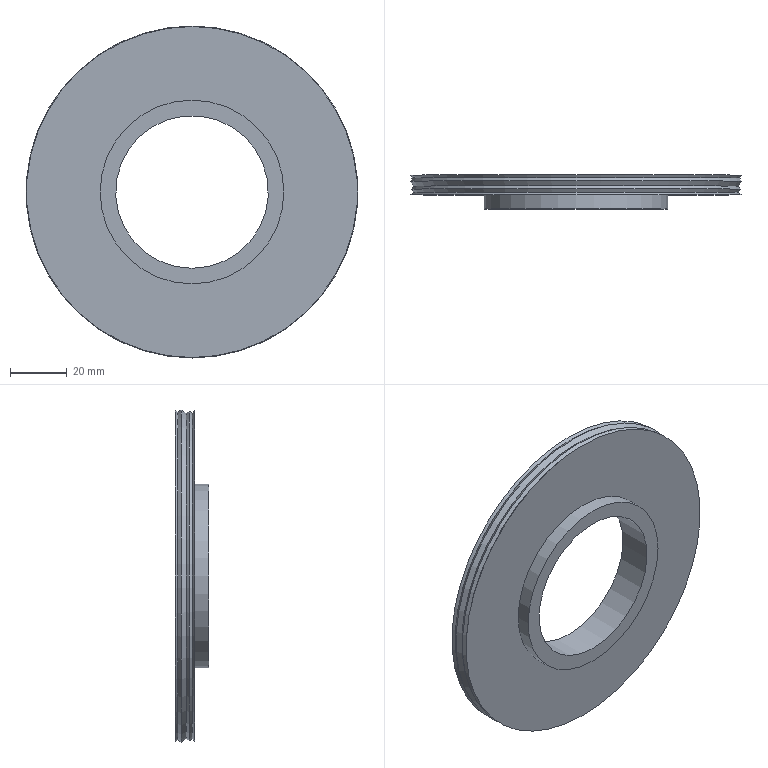Part | NX | features DATUM_CSYS 5, SKETCH 4, EXTRUDE 3, SWP104 1 | 1 solid | 11 faces | box 117.468 x 12 x 117.468 mm | volume 63462 mm3 | cone 6 | plane 3 | cylinder 2 | commonest cylinder face diameters 54 x1 65 x1
STEP:
#1=CARTESIAN_POINT('',(32.5,-7.,0.));
#2=VERTEX_POINT('',#1);
#3=CARTESIAN_POINT('',(0.,-7.,0.));
#4=DIRECTION('',(0.,-1.,0.));
#5=DIRECTION('',(1.,0.,0.));
#6=AXIS2_PLACEMENT_3D('',#3,#4,#5);
#7=CIRCLE('',#6,32.5);
#8=EDGE_CURVE('',#2,#2,#7,.T.);
#9=ORIENTED_EDGE('',*,*,#8,.F.);
#10=EDGE_LOOP('',(#9));
#11=FACE_BOUND('',#10,.T.);
#12=CARTESIAN_POINT('',(0.,-7.,-58.547));
#13=VERTEX_POINT('',#12);
#14=CARTESIAN_POINT('',(0.,-7.,0.));
#15=DIRECTION('',(0.,-1.,0.));
#16=DIRECTION('',(0.,0.,-1.));
#17=AXIS2_PLACEMENT_3D('',#14,#15,#16);
#18=CIRCLE('',#17,58.547);
#19=EDGE_CURVE('',#13,#13,#18,.T.);
#20=ORIENTED_EDGE('',*,*,#19,.T.);
#21=EDGE_LOOP('',(#20));
#22=FACE_BOUND('',#21,.T.);
#23=CARTESIAN_POINT('',(0.,-7.,0.));
#24=DIRECTION('',(0.,-1.,0.));
#25=DIRECTION('',(0.,0.,-1.));
#26=AXIS2_PLACEMENT_3D('',#23,#24,#25);
#27=PLANE('',#26);
#28=ADVANCED_FACE('',(#11,#22),#27,.T.);
#29=CARTESIAN_POINT('',(32.5,-12.,0.));
#30=VERTEX_POINT('',#29);
#31=CARTESIAN_POINT('',(0.,-12.,0.));
#32=DIRECTION('',(0.,-1.,0.));
#33=DIRECTION('',(1.,0.,0.));
#34=AXIS2_PLACEMENT_3D('',#31,#32,#33);
#35=CIRCLE('',#34,32.5);
#36=EDGE_CURVE('',#30,#30,#35,.T.);
#37=ORIENTED_EDGE('',*,*,#36,.F.);
#38=EDGE_LOOP('',(#37));
#39=FACE_BOUND('',#38,.T.);
#40=ORIENTED_EDGE('',*,*,#8,.T.);
#41=EDGE_LOOP('',(#40));
#42=FACE_BOUND('',#41,.T.);
#43=CARTESIAN_POINT('',(0.,-12.,0.));
#44=DIRECTION('',(0.,1.,0.));
#45=DIRECTION('',(0.,0.,1.));
#46=AXIS2_PLACEMENT_3D('',#43,#44,#45);
#47=CYLINDRICAL_SURFACE('',#46,32.5);
#48=ADVANCED_FACE('',(#39,#42),#47,.T.);
#49=CARTESIAN_POINT('',(0.,-12.,-27.));
#50=VERTEX_POINT('',#49);
#51=CARTESIAN_POINT('',(0.,-12.,0.));
#52=DIRECTION('',(0.,-1.,0.));
#53=DIRECTION('',(0.,0.,-1.));
#54=AXIS2_PLACEMENT_3D('',#51,#52,#53);
#55=CIRCLE('',#54,27.);
#56=EDGE_CURVE('',#50,#50,#55,.F.);
#57=ORIENTED_EDGE('',*,*,#56,.T.);
#58=EDGE_LOOP('',(#57));
#59=FACE_BOUND('',#58,.T.);
#60=ORIENTED_EDGE('',*,*,#36,.T.);
#61=EDGE_LOOP('',(#60));
#62=FACE_BOUND('',#61,.T.);
#63=CARTESIAN_POINT('',(0.,-12.,0.));
#64=DIRECTION('',(0.,-1.,0.));
#65=DIRECTION('',(0.,0.,-1.));
#66=AXIS2_PLACEMENT_3D('',#63,#64,#65);
#67=PLANE('',#66);
#68=ADVANCED_FACE('',(#59,#62),#67,.T.);
#69=CARTESIAN_POINT('',(0.,-1.,-58.));
#70=VERTEX_POINT('',#69);
#71=CARTESIAN_POINT('',(0.,-1.,0.));
#72=DIRECTION('',(0.,-1.,0.));
#73=DIRECTION('',(0.,0.,-1.));
#74=AXIS2_PLACEMENT_3D('',#71,#72,#73);
#75=CIRCLE('',#74,58.);
#76=EDGE_CURVE('',#70,#70,#75,.F.);
#77=ORIENTED_EDGE('',*,*,#76,.T.);
#78=EDGE_LOOP('',(#77));
#79=FACE_BOUND('',#78,.T.);
#80=CARTESIAN_POINT('',(0.,0.,-58.623));
#81=VERTEX_POINT('',#80);
#82=CARTESIAN_POINT('',(0.,0.,0.));
#83=DIRECTION('',(0.,-1.,0.));
#84=DIRECTION('',(0.,0.,-1.));
#85=AXIS2_PLACEMENT_3D('',#82,#83,#84);
#86=CIRCLE('',#85,58.623);
#87=EDGE_CURVE('',#81,#81,#86,.T.);
#88=ORIENTED_EDGE('',*,*,#87,.T.);
#89=EDGE_LOOP('',(#88));
#90=FACE_BOUND('',#89,.T.);
#91=CARTESIAN_POINT('',(0.,-1.,0.));
#92=DIRECTION('',(0.,1.,0.));
#93=DIRECTION('',(0.,0.,1.));
#94=AXIS2_PLACEMENT_3D('',#91,#92,#93);
#95=CONICAL_SURFACE('',#94,58.,0.5574);
#96=ADVANCED_FACE('',(#79,#90),#95,.T.);
#97=ORIENTED_EDGE('',*,*,#19,.F.);
#98=EDGE_LOOP('',(#97));
#99=FACE_BOUND('',#98,.T.);
#100=CARTESIAN_POINT('',(0.,-6.121,-57.586));
#101=VERTEX_POINT('',#100);
#102=CARTESIAN_POINT('',(0.,-6.121,0.));
#103=DIRECTION('',(0.,-1.,0.));
#104=DIRECTION('',(0.,0.,-1.));
#105=AXIS2_PLACEMENT_3D('',#102,#103,#104);
#106=CIRCLE('',#105,57.586);
#107=EDGE_CURVE('',#101,#101,#106,.F.);
#108=ORIENTED_EDGE('',*,*,#107,.F.);
#109=EDGE_LOOP('',(#108));
#110=FACE_BOUND('',#109,.T.);
#111=CARTESIAN_POINT('',(0.,-7.171,0.));
#112=DIRECTION('',(0.,-1.,0.));
#113=DIRECTION('',(0.,0.,-1.));
#114=AXIS2_PLACEMENT_3D('',#111,#112,#113);
#115=CONICAL_SURFACE('',#114,58.734,0.8299);
#116=ADVANCED_FACE('',(#99,#110),#115,.T.);
#117=CARTESIAN_POINT('',(0.,-4.953,-58.314));
#118=VERTEX_POINT('',#117);
#119=CARTESIAN_POINT('',(0.,-4.953,0.));
#120=DIRECTION('',(0.,-1.,0.));
#121=DIRECTION('',(0.,0.,-1.));
#122=AXIS2_PLACEMENT_3D('',#119,#120,#121);
#123=CIRCLE('',#122,58.314);
#124=EDGE_CURVE('',#118,#118,#123,.F.);
#125=ORIENTED_EDGE('',*,*,#124,.F.);
#126=EDGE_LOOP('',(#125));
#127=FACE_BOUND('',#126,.T.);
#128=ORIENTED_EDGE('',*,*,#107,.T.);
#129=EDGE_LOOP('',(#128));
#130=FACE_BOUND('',#129,.T.);
#131=CARTESIAN_POINT('',(0.,-6.121,0.));
#132=DIRECTION('',(0.,1.,0.));
#133=DIRECTION('',(0.,0.,1.));
#134=AXIS2_PLACEMENT_3D('',#131,#132,#133);
#135=CONICAL_SURFACE('',#134,57.586,0.5574);
#136=ADVANCED_FACE('',(#127,#130),#135,.T.);
#137=CARTESIAN_POINT('',(0.,-3.9,-57.631));
#138=VERTEX_POINT('',#137);
#139=CARTESIAN_POINT('',(0.,-3.9,0.));
#140=DIRECTION('',(0.,-1.,0.));
#141=DIRECTION('',(0.,0.,-1.));
#142=AXIS2_PLACEMENT_3D('',#139,#140,#141);
#143=CIRCLE('',#142,57.631);
#144=EDGE_CURVE('',#138,#138,#143,.F.);
#145=ORIENTED_EDGE('',*,*,#144,.F.);
#146=EDGE_LOOP('',(#145));
#147=FACE_BOUND('',#146,.T.);
#148=ORIENTED_EDGE('',*,*,#124,.T.);
#149=EDGE_LOOP('',(#148));
#150=FACE_BOUND('',#149,.T.);
#151=CARTESIAN_POINT('',(0.,-4.953,0.));
#152=DIRECTION('',(0.,-1.,0.));
#153=DIRECTION('',(0.,0.,-1.));
#154=AXIS2_PLACEMENT_3D('',#151,#152,#153);
#155=CONICAL_SURFACE('',#154,58.314,0.5756);
#156=ADVANCED_FACE('',(#147,#150),#155,.T.);
#157=CARTESIAN_POINT('',(0.,-2.131,-58.734));
#158=VERTEX_POINT('',#157);
#159=CARTESIAN_POINT('',(0.,-2.131,0.));
#160=DIRECTION('',(0.,-1.,0.));
#161=DIRECTION('',(0.,0.,-1.));
#162=AXIS2_PLACEMENT_3D('',#159,#160,#161);
#163=CIRCLE('',#162,58.734);
#164=EDGE_CURVE('',#158,#158,#163,.F.);
#165=ORIENTED_EDGE('',*,*,#164,.F.);
#166=EDGE_LOOP('',(#165));
#167=FACE_BOUND('',#166,.T.);
#168=ORIENTED_EDGE('',*,*,#144,.T.);
#169=EDGE_LOOP('',(#168));
#170=FACE_BOUND('',#169,.T.);
#171=CARTESIAN_POINT('',(0.,-3.9,0.));
#172=DIRECTION('',(0.,1.,0.));
#173=DIRECTION('',(0.,0.,1.));
#174=AXIS2_PLACEMENT_3D('',#171,#172,#173);
#175=CONICAL_SURFACE('',#174,57.631,0.5574);
#176=ADVANCED_FACE('',(#167,#170),#175,.T.);
#177=ORIENTED_EDGE('',*,*,#76,.F.);
#178=EDGE_LOOP('',(#177));
#179=FACE_BOUND('',#178,.T.);
#180=ORIENTED_EDGE('',*,*,#164,.T.);
#181=EDGE_LOOP('',(#180));
#182=FACE_BOUND('',#181,.T.);
#183=CARTESIAN_POINT('',(0.,-2.131,0.));
#184=DIRECTION('',(0.,-1.,0.));
#185=DIRECTION('',(0.,0.,-1.));
#186=AXIS2_PLACEMENT_3D('',#183,#184,#185);
#187=CONICAL_SURFACE('',#186,58.734,0.5756);
#188=ADVANCED_FACE('',(#179,#182),#187,.T.);
#189=CARTESIAN_POINT('',(0.,0.,-27.));
#190=VERTEX_POINT('',#189);
#191=CARTESIAN_POINT('',(0.,0.,0.));
#192=DIRECTION('',(0.,-1.,0.));
#193=DIRECTION('',(0.,0.,-1.));
#194=AXIS2_PLACEMENT_3D('',#191,#192,#193);
#195=CIRCLE('',#194,27.);
#196=EDGE_CURVE('',#190,#190,#195,.F.);
#197=ORIENTED_EDGE('',*,*,#196,.F.);
#198=EDGE_LOOP('',(#197));
#199=FACE_BOUND('',#198,.T.);
#200=ORIENTED_EDGE('',*,*,#87,.F.);
#201=EDGE_LOOP('',(#200));
#202=FACE_BOUND('',#201,.T.);
#203=CARTESIAN_POINT('',(0.,0.,0.));
#204=DIRECTION('',(0.,-1.,0.));
#205=DIRECTION('',(0.,0.,-1.));
#206=AXIS2_PLACEMENT_3D('',#203,#204,#205);
#207=PLANE('',#206);
#208=ADVANCED_FACE('',(#199,#202),#207,.F.);
#209=ORIENTED_EDGE('',*,*,#56,.F.);
#210=EDGE_LOOP('',(#209));
#211=FACE_BOUND('',#210,.T.);
#212=ORIENTED_EDGE('',*,*,#196,.T.);
#213=EDGE_LOOP('',(#212));
#214=FACE_BOUND('',#213,.T.);
#215=CARTESIAN_POINT('',(0.,-28.,0.));
#216=DIRECTION('',(0.,1.,0.));
#217=DIRECTION('',(0.,0.,1.));
#218=AXIS2_PLACEMENT_3D('',#215,#216,#217);
#219=CYLINDRICAL_SURFACE('',#218,27.);
#220=ADVANCED_FACE('',(#211,#214),#219,.F.);
#221=CLOSED_SHELL('',(#28,#48,#68,#96,#116,#136,#156,#176,#188,#208,#220));
#222=MANIFOLD_SOLID_BREP('',#221);
#223=(LENGTH_UNIT()NAMED_UNIT(*)SI_UNIT(.MILLI.,.METRE.));
#224=UNCERTAINTY_MEASURE_WITH_UNIT(LENGTH_MEASURE(0.00001),#223,'','');
#225=(NAMED_UNIT(*)PLANE_ANGLE_UNIT()SI_UNIT($,.RADIAN.));
#226=(NAMED_UNIT(*)SI_UNIT($,.STERADIAN.)SOLID_ANGLE_UNIT());
#227=(GEOMETRIC_REPRESENTATION_CONTEXT(3)GLOBAL_UNCERTAINTY_ASSIGNED_CONTEXT((#224))GLOBAL_UNIT_ASSIGNED_CONTEXT((#223,#225,#226))REPRESENTATION_CONTEXT('',''));
#228=ADVANCED_BREP_SHAPE_REPRESENTATION('',(#222),#227);